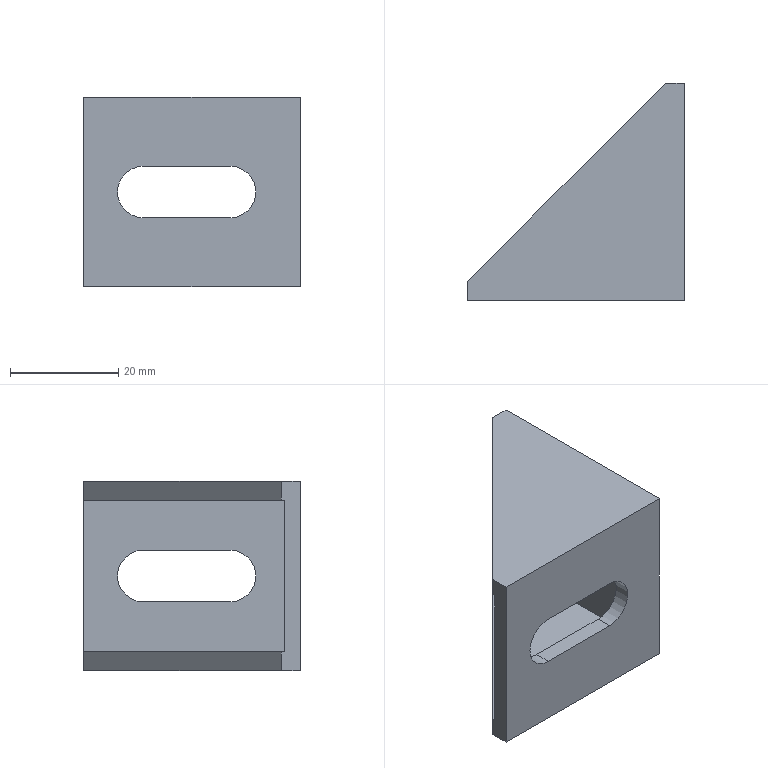Part | SolidWorks | features ICE 3, Extrusion 1 | 1 solid | 21 faces | box 40 x 40 x 35 mm | volume 11668 mm3 | plane 16 | cylinder 5 | commonest cylinder face diameters 9.5 x5
STEP:
#1=CARTESIAN_POINT('',(-16.25,0.,0.));
#2=VERTEX_POINT('',#1);
#3=CARTESIAN_POINT('',(-11.5,0.,4.75));
#4=VERTEX_POINT('',#3);
#5=CARTESIAN_POINT('',(-11.5,0.,0.));
#6=DIRECTION('',(0.,1.,0.));
#7=DIRECTION('',(-1.,0.,0.));
#8=AXIS2_PLACEMENT_3D('',#5,#6,#7);
#9=CIRCLE('',#8,4.75);
#10=EDGE_CURVE('',#2,#4,#9,.T.);
#11=ORIENTED_EDGE('',*,*,#10,.F.);
#12=CARTESIAN_POINT('',(-16.25,3.,0.));
#13=VERTEX_POINT('',#12);
#14=CARTESIAN_POINT('',(-16.25,0.,0.));
#15=DIRECTION('',(0.,1.,0.));
#16=VECTOR('',#15,1000.);
#17=LINE('',#14,#16);
#18=EDGE_CURVE('',#2,#13,#17,.T.);
#19=ORIENTED_EDGE('',*,*,#18,.T.);
#20=CARTESIAN_POINT('',(-11.5,3.,4.75));
#21=VERTEX_POINT('',#20);
#22=CARTESIAN_POINT('',(-11.5,3.,0.));
#23=DIRECTION('',(0.,1.,0.));
#24=DIRECTION('',(-1.,0.,0.));
#25=AXIS2_PLACEMENT_3D('',#22,#23,#24);
#26=CIRCLE('',#25,4.75);
#27=EDGE_CURVE('',#13,#21,#26,.T.);
#28=ORIENTED_EDGE('',*,*,#27,.T.);
#29=CARTESIAN_POINT('',(-11.5,0.,4.75));
#30=DIRECTION('',(0.,1.,0.));
#31=VECTOR('',#30,1000.);
#32=LINE('',#29,#31);
#33=EDGE_CURVE('',#4,#21,#32,.T.);
#34=ORIENTED_EDGE('',*,*,#33,.F.);
#35=EDGE_LOOP('',(#11,#19,#28,#34));
#36=FACE_OUTER_BOUND('',#35,.T.);
#37=CARTESIAN_POINT('',(-11.5,0.,0.));
#38=DIRECTION('',(0.,1.,0.));
#39=DIRECTION('',(-1.,0.,0.));
#40=AXIS2_PLACEMENT_3D('',#37,#38,#39);
#41=CYLINDRICAL_SURFACE('',#40,4.75);
#42=ADVANCED_FACE('',(#36),#41,.F.);
#43=CARTESIAN_POINT('',(14.,40.,14.));
#44=VERTEX_POINT('',#43);
#45=CARTESIAN_POINT('',(14.5,40.,14.));
#46=VERTEX_POINT('',#45);
#47=CARTESIAN_POINT('',(17.5,40.,14.));
#48=DIRECTION('',(1.,0.,0.));
#49=VECTOR('',#48,1000.);
#50=LINE('',#47,#49);
#51=EDGE_CURVE('',#44,#46,#50,.T.);
#52=ORIENTED_EDGE('',*,*,#51,.F.);
#53=CARTESIAN_POINT('',(14.,40.,17.5));
#54=VERTEX_POINT('',#53);
#55=CARTESIAN_POINT('',(14.,40.,17.5));
#56=DIRECTION('',(0.,0.,-1.));
#57=VECTOR('',#56,1000.);
#58=LINE('',#55,#57);
#59=EDGE_CURVE('',#54,#44,#58,.T.);
#60=ORIENTED_EDGE('',*,*,#59,.F.);
#61=CARTESIAN_POINT('',(17.5,40.,17.5));
#62=VERTEX_POINT('',#61);
#63=CARTESIAN_POINT('',(17.5,40.,17.5));
#64=DIRECTION('',(-1.,0.,0.));
#65=VECTOR('',#64,1000.);
#66=LINE('',#63,#65);
#67=EDGE_CURVE('',#62,#54,#66,.T.);
#68=ORIENTED_EDGE('',*,*,#67,.F.);
#69=CARTESIAN_POINT('',(17.5,40.,-17.5));
#70=VERTEX_POINT('',#69);
#71=CARTESIAN_POINT('',(17.5,40.,17.5));
#72=DIRECTION('',(0.,0.,-1.));
#73=VECTOR('',#72,1000.);
#74=LINE('',#71,#73);
#75=EDGE_CURVE('',#62,#70,#74,.T.);
#76=ORIENTED_EDGE('',*,*,#75,.T.);
#77=CARTESIAN_POINT('',(14.,40.,-17.5));
#78=VERTEX_POINT('',#77);
#79=CARTESIAN_POINT('',(17.5,40.,-17.5));
#80=DIRECTION('',(-1.,0.,0.));
#81=VECTOR('',#80,1000.);
#82=LINE('',#79,#81);
#83=EDGE_CURVE('',#70,#78,#82,.T.);
#84=ORIENTED_EDGE('',*,*,#83,.T.);
#85=CARTESIAN_POINT('',(14.,40.,-14.));
#86=VERTEX_POINT('',#85);
#87=CARTESIAN_POINT('',(14.,40.,17.5));
#88=DIRECTION('',(0.,0.,-1.));
#89=VECTOR('',#88,1000.);
#90=LINE('',#87,#89);
#91=EDGE_CURVE('',#86,#78,#90,.T.);
#92=ORIENTED_EDGE('',*,*,#91,.F.);
#93=CARTESIAN_POINT('',(14.5,40.,-14.));
#94=VERTEX_POINT('',#93);
#95=CARTESIAN_POINT('',(17.5,40.,-14.));
#96=DIRECTION('',(1.,0.,0.));
#97=VECTOR('',#96,1000.);
#98=LINE('',#95,#97);
#99=EDGE_CURVE('',#86,#94,#98,.T.);
#100=ORIENTED_EDGE('',*,*,#99,.T.);
#101=CARTESIAN_POINT('',(14.5,40.,17.5));
#102=DIRECTION('',(0.,0.,-1.));
#103=VECTOR('',#102,1000.);
#104=LINE('',#101,#103);
#105=EDGE_CURVE('',#46,#94,#104,.T.);
#106=ORIENTED_EDGE('',*,*,#105,.F.);
#107=EDGE_LOOP('',(#52,#60,#68,#76,#84,#92,#100,#106));
#108=FACE_OUTER_BOUND('',#107,.T.);
#109=CARTESIAN_POINT('',(17.5,40.,17.5));
#110=DIRECTION('',(0.,-1.,0.));
#111=DIRECTION('',(0.,0.,-1.));
#112=AXIS2_PLACEMENT_3D('',#109,#110,#111);
#113=PLANE('',#112);
#114=ADVANCED_FACE('',(#108),#113,.F.);
#115=CARTESIAN_POINT('',(-22.5,3.5,14.));
#116=VERTEX_POINT('',#115);
#117=CARTESIAN_POINT('',(14.,40.,14.));
#118=DIRECTION('',(0.7071,0.7071,0.));
#119=VECTOR('',#118,1000.);
#120=LINE('',#117,#119);
#121=EDGE_CURVE('',#116,#44,#120,.T.);
#122=ORIENTED_EDGE('',*,*,#121,.F.);
#123=CARTESIAN_POINT('',(-22.5,3.5,17.5));
#124=VERTEX_POINT('',#123);
#125=CARTESIAN_POINT('',(-22.5,3.5,17.5));
#126=DIRECTION('',(0.,0.,-1.));
#127=VECTOR('',#126,1000.);
#128=LINE('',#125,#127);
#129=EDGE_CURVE('',#124,#116,#128,.T.);
#130=ORIENTED_EDGE('',*,*,#129,.F.);
#131=CARTESIAN_POINT('',(14.,40.,17.5));
#132=DIRECTION('',(-0.7071,-0.7071,0.));
#133=VECTOR('',#132,1000.);
#134=LINE('',#131,#133);
#135=EDGE_CURVE('',#54,#124,#134,.T.);
#136=ORIENTED_EDGE('',*,*,#135,.F.);
#137=ORIENTED_EDGE('',*,*,#59,.T.);
#138=EDGE_LOOP('',(#122,#130,#136,#137));
#139=FACE_OUTER_BOUND('',#138,.T.);
#140=CARTESIAN_POINT('',(14.,40.,17.5));
#141=DIRECTION('',(0.7071,-0.7071,0.));
#142=DIRECTION('',(0.7071,0.7071,0.));
#143=AXIS2_PLACEMENT_3D('',#140,#141,#142);
#144=PLANE('',#143);
#145=ADVANCED_FACE('',(#139),#144,.F.);
#146=CARTESIAN_POINT('',(-22.5,3.,14.));
#147=VERTEX_POINT('',#146);
#148=CARTESIAN_POINT('',(-22.5,0.,14.));
#149=DIRECTION('',(0.,1.,0.));
#150=VECTOR('',#149,1000.);
#151=LINE('',#148,#150);
#152=EDGE_CURVE('',#147,#116,#151,.T.);
#153=ORIENTED_EDGE('',*,*,#152,.F.);
#154=CARTESIAN_POINT('',(-22.5,3.,-14.));
#155=VERTEX_POINT('',#154);
#156=CARTESIAN_POINT('',(-22.5,3.,17.5));
#157=DIRECTION('',(0.,0.,1.));
#158=VECTOR('',#157,1000.);
#159=LINE('',#156,#158);
#160=EDGE_CURVE('',#155,#147,#159,.T.);
#161=ORIENTED_EDGE('',*,*,#160,.F.);
#162=CARTESIAN_POINT('',(-22.5,3.5,-14.));
#163=VERTEX_POINT('',#162);
#164=CARTESIAN_POINT('',(-22.5,0.,-14.));
#165=DIRECTION('',(0.,1.,0.));
#166=VECTOR('',#165,1000.);
#167=LINE('',#164,#166);
#168=EDGE_CURVE('',#155,#163,#167,.T.);
#169=ORIENTED_EDGE('',*,*,#168,.T.);
#170=CARTESIAN_POINT('',(-22.5,3.5,-17.5));
#171=VERTEX_POINT('',#170);
#172=CARTESIAN_POINT('',(-22.5,3.5,17.5));
#173=DIRECTION('',(0.,0.,-1.));
#174=VECTOR('',#173,1000.);
#175=LINE('',#172,#174);
#176=EDGE_CURVE('',#163,#171,#175,.T.);
#177=ORIENTED_EDGE('',*,*,#176,.T.);
#178=CARTESIAN_POINT('',(-22.5,0.,-17.5));
#179=VERTEX_POINT('',#178);
#180=CARTESIAN_POINT('',(-22.5,0.,-17.5));
#181=DIRECTION('',(0.,-1.,0.));
#182=VECTOR('',#181,1000.);
#183=LINE('',#180,#182);
#184=EDGE_CURVE('',#171,#179,#183,.T.);
#185=ORIENTED_EDGE('',*,*,#184,.T.);
#186=CARTESIAN_POINT('',(-22.5,0.,17.5));
#187=VERTEX_POINT('',#186);
#188=CARTESIAN_POINT('',(-22.5,0.,17.5));
#189=DIRECTION('',(0.,0.,-1.));
#190=VECTOR('',#189,1000.);
#191=LINE('',#188,#190);
#192=EDGE_CURVE('',#187,#179,#191,.T.);
#193=ORIENTED_EDGE('',*,*,#192,.F.);
#194=CARTESIAN_POINT('',(-22.5,0.,17.5));
#195=DIRECTION('',(0.,-1.,0.));
#196=VECTOR('',#195,1000.);
#197=LINE('',#194,#196);
#198=EDGE_CURVE('',#124,#187,#197,.T.);
#199=ORIENTED_EDGE('',*,*,#198,.F.);
#200=ORIENTED_EDGE('',*,*,#129,.T.);
#201=EDGE_LOOP('',(#153,#161,#169,#177,#185,#193,#199,#200));
#202=FACE_OUTER_BOUND('',#201,.T.);
#203=CARTESIAN_POINT('',(-22.5,0.,17.5));
#204=DIRECTION('',(1.,0.,0.));
#205=DIRECTION('',(0.,0.,-1.));
#206=AXIS2_PLACEMENT_3D('',#203,#204,#205);
#207=PLANE('',#206);
#208=ADVANCED_FACE('',(#202),#207,.F.);
#209=CARTESIAN_POINT('',(17.5,29.,-4.75));
#210=VERTEX_POINT('',#209);
#211=CARTESIAN_POINT('',(17.5,13.,-4.75));
#212=VERTEX_POINT('',#211);
#213=CARTESIAN_POINT('',(17.5,13.,-4.75));
#214=DIRECTION('',(0.,-1.,0.));
#215=VECTOR('',#214,1000.);
#216=LINE('',#213,#215);
#217=EDGE_CURVE('',#210,#212,#216,.T.);
#218=ORIENTED_EDGE('',*,*,#217,.T.);
#219=CARTESIAN_POINT('',(17.5,13.,4.75));
#220=VERTEX_POINT('',#219);
#221=CARTESIAN_POINT('',(17.5,13.,0.));
#222=DIRECTION('',(-1.,0.,0.));
#223=DIRECTION('',(0.,0.,1.));
#224=AXIS2_PLACEMENT_3D('',#221,#222,#223);
#225=CIRCLE('',#224,4.75);
#226=EDGE_CURVE('',#212,#220,#225,.T.);
#227=ORIENTED_EDGE('',*,*,#226,.T.);
#228=CARTESIAN_POINT('',(17.5,29.,4.75));
#229=VERTEX_POINT('',#228);
#230=CARTESIAN_POINT('',(17.5,13.,4.75));
#231=DIRECTION('',(0.,1.,0.));
#232=VECTOR('',#231,1000.);
#233=LINE('',#230,#232);
#234=EDGE_CURVE('',#220,#229,#233,.T.);
#235=ORIENTED_EDGE('',*,*,#234,.T.);
#236=CARTESIAN_POINT('',(17.5,29.,0.));
#237=DIRECTION('',(-1.,0.,0.));
#238=DIRECTION('',(0.,0.,1.));
#239=AXIS2_PLACEMENT_3D('',#236,#237,#238);
#240=CIRCLE('',#239,4.75);
#241=EDGE_CURVE('',#229,#210,#240,.T.);
#242=ORIENTED_EDGE('',*,*,#241,.T.);
#243=EDGE_LOOP('',(#218,#227,#235,#242));
#244=FACE_BOUND('',#243,.T.);
#245=CARTESIAN_POINT('',(17.5,0.,-17.5));
#246=VERTEX_POINT('',#245);
#247=CARTESIAN_POINT('',(17.5,0.,-17.5));
#248=DIRECTION('',(0.,1.,0.));
#249=VECTOR('',#248,1000.);
#250=LINE('',#247,#249);
#251=EDGE_CURVE('',#246,#70,#250,.T.);
#252=ORIENTED_EDGE('',*,*,#251,.T.);
#253=ORIENTED_EDGE('',*,*,#75,.F.);
#254=CARTESIAN_POINT('',(17.5,0.,17.5));
#255=VERTEX_POINT('',#254);
#256=CARTESIAN_POINT('',(17.5,0.,17.5));
#257=DIRECTION('',(0.,1.,0.));
#258=VECTOR('',#257,1000.);
#259=LINE('',#256,#258);
#260=EDGE_CURVE('',#255,#62,#259,.T.);
#261=ORIENTED_EDGE('',*,*,#260,.F.);
#262=CARTESIAN_POINT('',(17.5,0.,17.5));
#263=DIRECTION('',(0.,0.,-1.));
#264=VECTOR('',#263,1000.);
#265=LINE('',#262,#264);
#266=EDGE_CURVE('',#255,#246,#265,.T.);
#267=ORIENTED_EDGE('',*,*,#266,.T.);
#268=EDGE_LOOP('',(#252,#253,#261,#267));
#269=FACE_OUTER_BOUND('',#268,.T.);
#270=CARTESIAN_POINT('',(17.5,0.,17.5));
#271=DIRECTION('',(-1.,0.,0.));
#272=DIRECTION('',(0.,0.,1.));
#273=AXIS2_PLACEMENT_3D('',#270,#271,#272);
#274=PLANE('',#273);
#275=ADVANCED_FACE('',(#244,#269),#274,.F.);
#276=ORIENTED_EDGE('',*,*,#176,.F.);
#277=CARTESIAN_POINT('',(14.,40.,-14.));
#278=DIRECTION('',(0.7071,0.7071,0.));
#279=VECTOR('',#278,1000.);
#280=LINE('',#277,#279);
#281=EDGE_CURVE('',#163,#86,#280,.T.);
#282=ORIENTED_EDGE('',*,*,#281,.T.);
#283=ORIENTED_EDGE('',*,*,#91,.T.);
#284=CARTESIAN_POINT('',(14.,40.,-17.5));
#285=DIRECTION('',(-0.7071,-0.7071,0.));
#286=VECTOR('',#285,1000.);
#287=LINE('',#284,#286);
#288=EDGE_CURVE('',#78,#171,#287,.T.);
#289=ORIENTED_EDGE('',*,*,#288,.T.);
#290=EDGE_LOOP('',(#276,#282,#283,#289));
#291=FACE_OUTER_BOUND('',#290,.T.);
#292=CARTESIAN_POINT('',(14.,40.,17.5));
#293=DIRECTION('',(0.7071,-0.7071,0.));
#294=DIRECTION('',(0.7071,0.7071,0.));
#295=AXIS2_PLACEMENT_3D('',#292,#293,#294);
#296=PLANE('',#295);
#297=ADVANCED_FACE('',(#291),#296,.F.);
#298=CARTESIAN_POINT('',(4.5,0.,-4.75));
#299=VERTEX_POINT('',#298);
#300=CARTESIAN_POINT('',(-11.5,0.,-4.75));
#301=VERTEX_POINT('',#300);
#302=CARTESIAN_POINT('',(-11.5,0.,-4.75));
#303=DIRECTION('',(-1.,0.,0.));
#304=VECTOR('',#303,1000.);
#305=LINE('',#302,#304);
#306=EDGE_CURVE('',#299,#301,#305,.T.);
#307=ORIENTED_EDGE('',*,*,#306,.T.);
#308=CARTESIAN_POINT('',(-11.5,0.,0.));
#309=DIRECTION('',(0.,1.,0.));
#310=DIRECTION('',(-1.,0.,0.));
#311=AXIS2_PLACEMENT_3D('',#308,#309,#310);
#312=CIRCLE('',#311,4.75);
#313=EDGE_CURVE('',#301,#2,#312,.T.);
#314=ORIENTED_EDGE('',*,*,#313,.T.);
#315=ORIENTED_EDGE('',*,*,#10,.T.);
#316=CARTESIAN_POINT('',(4.5,0.,4.75));
#317=VERTEX_POINT('',#316);
#318=CARTESIAN_POINT('',(-11.5,0.,4.75));
#319=DIRECTION('',(1.,0.,0.));
#320=VECTOR('',#319,1000.);
#321=LINE('',#318,#320);
#322=EDGE_CURVE('',#4,#317,#321,.T.);
#323=ORIENTED_EDGE('',*,*,#322,.T.);
#324=CARTESIAN_POINT('',(4.5,0.,0.));
#325=DIRECTION('',(0.,1.,0.));
#326=DIRECTION('',(-1.,0.,0.));
#327=AXIS2_PLACEMENT_3D('',#324,#325,#326);
#328=CIRCLE('',#327,4.75);
#329=EDGE_CURVE('',#317,#299,#328,.T.);
#330=ORIENTED_EDGE('',*,*,#329,.T.);
#331=EDGE_LOOP('',(#307,#314,#315,#323,#330));
#332=FACE_BOUND('',#331,.T.);
#333=CARTESIAN_POINT('',(-22.5,0.,-17.5));
#334=DIRECTION('',(1.,0.,0.));
#335=VECTOR('',#334,1000.);
#336=LINE('',#333,#335);
#337=EDGE_CURVE('',#179,#246,#336,.T.);
#338=ORIENTED_EDGE('',*,*,#337,.T.);
#339=ORIENTED_EDGE('',*,*,#266,.F.);
#340=CARTESIAN_POINT('',(-22.5,0.,17.5));
#341=DIRECTION('',(1.,0.,0.));
#342=VECTOR('',#341,1000.);
#343=LINE('',#340,#342);
#344=EDGE_CURVE('',#187,#255,#343,.T.);
#345=ORIENTED_EDGE('',*,*,#344,.F.);
#346=ORIENTED_EDGE('',*,*,#192,.T.);
#347=EDGE_LOOP('',(#338,#339,#345,#346));
#348=FACE_OUTER_BOUND('',#347,.T.);
#349=CARTESIAN_POINT('',(-22.5,0.,17.5));
#350=DIRECTION('',(0.,1.,0.));
#351=DIRECTION('',(0.,0.,1.));
#352=AXIS2_PLACEMENT_3D('',#349,#350,#351);
#353=PLANE('',#352);
#354=ADVANCED_FACE('',(#332,#348),#353,.F.);
#355=ORIENTED_EDGE('',*,*,#260,.T.);
#356=ORIENTED_EDGE('',*,*,#67,.T.);
#357=ORIENTED_EDGE('',*,*,#135,.T.);
#358=ORIENTED_EDGE('',*,*,#198,.T.);
#359=ORIENTED_EDGE('',*,*,#344,.T.);
#360=EDGE_LOOP('',(#355,#356,#357,#358,#359));
#361=FACE_OUTER_BOUND('',#360,.T.);
#362=CARTESIAN_POINT('',(0.,0.,17.5));
#363=DIRECTION('',(0.,0.,1.));
#364=DIRECTION('',(1.,0.,0.));
#365=AXIS2_PLACEMENT_3D('',#362,#363,#364);
#366=PLANE('',#365);
#367=ADVANCED_FACE('',(#361),#366,.T.);
#368=ORIENTED_EDGE('',*,*,#251,.F.);
#369=ORIENTED_EDGE('',*,*,#337,.F.);
#370=ORIENTED_EDGE('',*,*,#184,.F.);
#371=ORIENTED_EDGE('',*,*,#288,.F.);
#372=ORIENTED_EDGE('',*,*,#83,.F.);
#373=EDGE_LOOP('',(#368,#369,#370,#371,#372));
#374=FACE_OUTER_BOUND('',#373,.T.);
#375=CARTESIAN_POINT('',(0.,0.,-17.5));
#376=DIRECTION('',(0.,0.,1.));
#377=DIRECTION('',(1.,0.,0.));
#378=AXIS2_PLACEMENT_3D('',#375,#376,#377);
#379=PLANE('',#378);
#380=ADVANCED_FACE('',(#374),#379,.F.);
#381=CARTESIAN_POINT('',(14.5,13.,-4.75));
#382=VERTEX_POINT('',#381);
#383=CARTESIAN_POINT('',(14.5,13.,4.75));
#384=VERTEX_POINT('',#383);
#385=CARTESIAN_POINT('',(14.5,13.,0.));
#386=DIRECTION('',(-1.,0.,0.));
#387=DIRECTION('',(0.,0.,1.));
#388=AXIS2_PLACEMENT_3D('',#385,#386,#387);
#389=CIRCLE('',#388,4.75);
#390=EDGE_CURVE('',#382,#384,#389,.T.);
#391=ORIENTED_EDGE('',*,*,#390,.F.);
#392=CARTESIAN_POINT('',(14.5,29.,-4.75));
#393=VERTEX_POINT('',#392);
#394=CARTESIAN_POINT('',(14.5,13.,-4.75));
#395=DIRECTION('',(0.,-1.,0.));
#396=VECTOR('',#395,1000.);
#397=LINE('',#394,#396);
#398=EDGE_CURVE('',#393,#382,#397,.T.);
#399=ORIENTED_EDGE('',*,*,#398,.F.);
#400=CARTESIAN_POINT('',(14.5,29.,4.75));
#401=VERTEX_POINT('',#400);
#402=CARTESIAN_POINT('',(14.5,29.,0.));
#403=DIRECTION('',(-1.,0.,0.));
#404=DIRECTION('',(0.,0.,1.));
#405=AXIS2_PLACEMENT_3D('',#402,#403,#404);
#406=CIRCLE('',#405,4.75);
#407=EDGE_CURVE('',#401,#393,#406,.T.);
#408=ORIENTED_EDGE('',*,*,#407,.F.);
#409=CARTESIAN_POINT('',(14.5,13.,4.75));
#410=DIRECTION('',(0.,1.,0.));
#411=VECTOR('',#410,1000.);
#412=LINE('',#409,#411);
#413=EDGE_CURVE('',#384,#401,#412,.T.);
#414=ORIENTED_EDGE('',*,*,#413,.F.);
#415=EDGE_LOOP('',(#391,#399,#408,#414));
#416=FACE_BOUND('',#415,.T.);
#417=ORIENTED_EDGE('',*,*,#105,.T.);
#418=CARTESIAN_POINT('',(14.5,3.,-14.));
#419=VERTEX_POINT('',#418);
#420=CARTESIAN_POINT('',(14.5,3.,-14.));
#421=DIRECTION('',(0.,1.,0.));
#422=VECTOR('',#421,1000.);
#423=LINE('',#420,#422);
#424=EDGE_CURVE('',#419,#94,#423,.T.);
#425=ORIENTED_EDGE('',*,*,#424,.F.);
#426=CARTESIAN_POINT('',(14.5,3.,14.));
#427=VERTEX_POINT('',#426);
#428=CARTESIAN_POINT('',(14.5,3.,14.));
#429=DIRECTION('',(0.,0.,-1.));
#430=VECTOR('',#429,1000.);
#431=LINE('',#428,#430);
#432=EDGE_CURVE('',#427,#419,#431,.T.);
#433=ORIENTED_EDGE('',*,*,#432,.F.);
#434=CARTESIAN_POINT('',(14.5,3.,14.));
#435=DIRECTION('',(0.,1.,0.));
#436=VECTOR('',#435,1000.);
#437=LINE('',#434,#436);
#438=EDGE_CURVE('',#427,#46,#437,.T.);
#439=ORIENTED_EDGE('',*,*,#438,.T.);
#440=EDGE_LOOP('',(#417,#425,#433,#439));
#441=FACE_OUTER_BOUND('',#440,.T.);
#442=CARTESIAN_POINT('',(14.5,3.,14.));
#443=DIRECTION('',(-1.,0.,0.));
#444=DIRECTION('',(0.,0.,1.));
#445=AXIS2_PLACEMENT_3D('',#442,#443,#444);
#446=PLANE('',#445);
#447=ADVANCED_FACE('',(#416,#441),#446,.T.);
#448=CARTESIAN_POINT('',(-11.5,3.,-4.75));
#449=VERTEX_POINT('',#448);
#450=CARTESIAN_POINT('',(-11.5,3.,0.));
#451=DIRECTION('',(0.,1.,0.));
#452=DIRECTION('',(-1.,0.,0.));
#453=AXIS2_PLACEMENT_3D('',#450,#451,#452);
#454=CIRCLE('',#453,4.75);
#455=EDGE_CURVE('',#449,#13,#454,.T.);
#456=ORIENTED_EDGE('',*,*,#455,.F.);
#457=CARTESIAN_POINT('',(4.5,3.,-4.75));
#458=VERTEX_POINT('',#457);
#459=CARTESIAN_POINT('',(-11.5,3.,-4.75));
#460=DIRECTION('',(-1.,0.,0.));
#461=VECTOR('',#460,1000.);
#462=LINE('',#459,#461);
#463=EDGE_CURVE('',#458,#449,#462,.T.);
#464=ORIENTED_EDGE('',*,*,#463,.F.);
#465=CARTESIAN_POINT('',(4.5,3.,4.75));
#466=VERTEX_POINT('',#465);
#467=CARTESIAN_POINT('',(4.5,3.,0.));
#468=DIRECTION('',(0.,1.,0.));
#469=DIRECTION('',(-1.,0.,0.));
#470=AXIS2_PLACEMENT_3D('',#467,#468,#469);
#471=CIRCLE('',#470,4.75);
#472=EDGE_CURVE('',#466,#458,#471,.T.);
#473=ORIENTED_EDGE('',*,*,#472,.F.);
#474=CARTESIAN_POINT('',(-11.5,3.,4.75));
#475=DIRECTION('',(1.,0.,0.));
#476=VECTOR('',#475,1000.);
#477=LINE('',#474,#476);
#478=EDGE_CURVE('',#21,#466,#477,.T.);
#479=ORIENTED_EDGE('',*,*,#478,.F.);
#480=ORIENTED_EDGE('',*,*,#27,.F.);
#481=EDGE_LOOP('',(#456,#464,#473,#479,#480));
#482=FACE_BOUND('',#481,.T.);
#483=ORIENTED_EDGE('',*,*,#160,.T.);
#484=CARTESIAN_POINT('',(-34.195,3.,14.));
#485=DIRECTION('',(1.,0.,0.));
#486=VECTOR('',#485,1000.);
#487=LINE('',#484,#486);
#488=EDGE_CURVE('',#147,#427,#487,.T.);
#489=ORIENTED_EDGE('',*,*,#488,.T.);
#490=ORIENTED_EDGE('',*,*,#432,.T.);
#491=CARTESIAN_POINT('',(-34.195,3.,-14.));
#492=DIRECTION('',(1.,0.,0.));
#493=VECTOR('',#492,1000.);
#494=LINE('',#491,#493);
#495=EDGE_CURVE('',#155,#419,#494,.T.);
#496=ORIENTED_EDGE('',*,*,#495,.F.);
#497=EDGE_LOOP('',(#483,#489,#490,#496));
#498=FACE_OUTER_BOUND('',#497,.T.);
#499=CARTESIAN_POINT('',(-34.195,3.,14.));
#500=DIRECTION('',(0.,1.,0.));
#501=DIRECTION('',(-1.,0.,0.));
#502=AXIS2_PLACEMENT_3D('',#499,#500,#501);
#503=PLANE('',#502);
#504=ADVANCED_FACE('',(#482,#498),#503,.T.);
#505=ORIENTED_EDGE('',*,*,#51,.T.);
#506=ORIENTED_EDGE('',*,*,#438,.F.);
#507=ORIENTED_EDGE('',*,*,#488,.F.);
#508=ORIENTED_EDGE('',*,*,#152,.T.);
#509=ORIENTED_EDGE('',*,*,#121,.T.);
#510=EDGE_LOOP('',(#505,#506,#507,#508,#509));
#511=FACE_OUTER_BOUND('',#510,.T.);
#512=CARTESIAN_POINT('',(0.,0.,14.));
#513=DIRECTION('',(0.,0.,-1.));
#514=DIRECTION('',(-1.,0.,0.));
#515=AXIS2_PLACEMENT_3D('',#512,#513,#514);
#516=PLANE('',#515);
#517=ADVANCED_FACE('',(#511),#516,.T.);
#518=ORIENTED_EDGE('',*,*,#281,.F.);
#519=ORIENTED_EDGE('',*,*,#168,.F.);
#520=ORIENTED_EDGE('',*,*,#495,.T.);
#521=ORIENTED_EDGE('',*,*,#424,.T.);
#522=ORIENTED_EDGE('',*,*,#99,.F.);
#523=EDGE_LOOP('',(#518,#519,#520,#521,#522));
#524=FACE_OUTER_BOUND('',#523,.T.);
#525=CARTESIAN_POINT('',(0.,0.,-14.));
#526=DIRECTION('',(0.,0.,-1.));
#527=DIRECTION('',(-1.,0.,0.));
#528=AXIS2_PLACEMENT_3D('',#525,#526,#527);
#529=PLANE('',#528);
#530=ADVANCED_FACE('',(#524),#529,.F.);
#531=ORIENTED_EDGE('',*,*,#18,.F.);
#532=ORIENTED_EDGE('',*,*,#313,.F.);
#533=CARTESIAN_POINT('',(-11.5,0.,-4.75));
#534=DIRECTION('',(0.,1.,0.));
#535=VECTOR('',#534,1000.);
#536=LINE('',#533,#535);
#537=EDGE_CURVE('',#301,#449,#536,.T.);
#538=ORIENTED_EDGE('',*,*,#537,.T.);
#539=ORIENTED_EDGE('',*,*,#455,.T.);
#540=EDGE_LOOP('',(#531,#532,#538,#539));
#541=FACE_OUTER_BOUND('',#540,.T.);
#542=CARTESIAN_POINT('',(-11.5,0.,0.));
#543=DIRECTION('',(0.,1.,0.));
#544=DIRECTION('',(-1.,0.,0.));
#545=AXIS2_PLACEMENT_3D('',#542,#543,#544);
#546=CYLINDRICAL_SURFACE('',#545,4.75);
#547=ADVANCED_FACE('',(#541),#546,.F.);
#548=ORIENTED_EDGE('',*,*,#463,.T.);
#549=ORIENTED_EDGE('',*,*,#537,.F.);
#550=ORIENTED_EDGE('',*,*,#306,.F.);
#551=CARTESIAN_POINT('',(4.5,0.,-4.75));
#552=DIRECTION('',(0.,1.,0.));
#553=VECTOR('',#552,1000.);
#554=LINE('',#551,#553);
#555=EDGE_CURVE('',#299,#458,#554,.T.);
#556=ORIENTED_EDGE('',*,*,#555,.T.);
#557=EDGE_LOOP('',(#548,#549,#550,#556));
#558=FACE_OUTER_BOUND('',#557,.T.);
#559=CARTESIAN_POINT('',(-11.5,0.,-4.75));
#560=DIRECTION('',(0.,0.,-1.));
#561=DIRECTION('',(-1.,0.,0.));
#562=AXIS2_PLACEMENT_3D('',#559,#560,#561);
#563=PLANE('',#562);
#564=ADVANCED_FACE('',(#558),#563,.F.);
#565=ORIENTED_EDGE('',*,*,#472,.T.);
#566=ORIENTED_EDGE('',*,*,#555,.F.);
#567=ORIENTED_EDGE('',*,*,#329,.F.);
#568=CARTESIAN_POINT('',(4.5,0.,4.75));
#569=DIRECTION('',(0.,1.,0.));
#570=VECTOR('',#569,1000.);
#571=LINE('',#568,#570);
#572=EDGE_CURVE('',#317,#466,#571,.T.);
#573=ORIENTED_EDGE('',*,*,#572,.T.);
#574=EDGE_LOOP('',(#565,#566,#567,#573));
#575=FACE_OUTER_BOUND('',#574,.T.);
#576=CARTESIAN_POINT('',(4.5,0.,0.));
#577=DIRECTION('',(0.,1.,0.));
#578=DIRECTION('',(-1.,0.,0.));
#579=AXIS2_PLACEMENT_3D('',#576,#577,#578);
#580=CYLINDRICAL_SURFACE('',#579,4.75);
#581=ADVANCED_FACE('',(#575),#580,.F.);
#582=ORIENTED_EDGE('',*,*,#478,.T.);
#583=ORIENTED_EDGE('',*,*,#572,.F.);
#584=ORIENTED_EDGE('',*,*,#322,.F.);
#585=ORIENTED_EDGE('',*,*,#33,.T.);
#586=EDGE_LOOP('',(#582,#583,#584,#585));
#587=FACE_OUTER_BOUND('',#586,.T.);
#588=CARTESIAN_POINT('',(-11.5,0.,4.75));
#589=DIRECTION('',(0.,0.,1.));
#590=DIRECTION('',(1.,0.,0.));
#591=AXIS2_PLACEMENT_3D('',#588,#589,#590);
#592=PLANE('',#591);
#593=ADVANCED_FACE('',(#587),#592,.F.);
#594=ORIENTED_EDGE('',*,*,#390,.T.);
#595=CARTESIAN_POINT('',(17.5,13.,4.75));
#596=DIRECTION('',(-1.,0.,0.));
#597=VECTOR('',#596,1000.);
#598=LINE('',#595,#597);
#599=EDGE_CURVE('',#220,#384,#598,.T.);
#600=ORIENTED_EDGE('',*,*,#599,.F.);
#601=ORIENTED_EDGE('',*,*,#226,.F.);
#602=CARTESIAN_POINT('',(17.5,13.,-4.75));
#603=DIRECTION('',(-1.,0.,0.));
#604=VECTOR('',#603,1000.);
#605=LINE('',#602,#604);
#606=EDGE_CURVE('',#212,#382,#605,.T.);
#607=ORIENTED_EDGE('',*,*,#606,.T.);
#608=EDGE_LOOP('',(#594,#600,#601,#607));
#609=FACE_OUTER_BOUND('',#608,.T.);
#610=CARTESIAN_POINT('',(17.5,13.,0.));
#611=DIRECTION('',(-1.,0.,0.));
#612=DIRECTION('',(0.,0.,1.));
#613=AXIS2_PLACEMENT_3D('',#610,#611,#612);
#614=CYLINDRICAL_SURFACE('',#613,4.75);
#615=ADVANCED_FACE('',(#609),#614,.F.);
#616=ORIENTED_EDGE('',*,*,#398,.T.);
#617=ORIENTED_EDGE('',*,*,#606,.F.);
#618=ORIENTED_EDGE('',*,*,#217,.F.);
#619=CARTESIAN_POINT('',(17.5,29.,-4.75));
#620=DIRECTION('',(-1.,0.,0.));
#621=VECTOR('',#620,1000.);
#622=LINE('',#619,#621);
#623=EDGE_CURVE('',#210,#393,#622,.T.);
#624=ORIENTED_EDGE('',*,*,#623,.T.);
#625=EDGE_LOOP('',(#616,#617,#618,#624));
#626=FACE_OUTER_BOUND('',#625,.T.);
#627=CARTESIAN_POINT('',(17.5,13.,-4.75));
#628=DIRECTION('',(0.,0.,-1.));
#629=DIRECTION('',(-1.,0.,0.));
#630=AXIS2_PLACEMENT_3D('',#627,#628,#629);
#631=PLANE('',#630);
#632=ADVANCED_FACE('',(#626),#631,.F.);
#633=ORIENTED_EDGE('',*,*,#407,.T.);
#634=ORIENTED_EDGE('',*,*,#623,.F.);
#635=ORIENTED_EDGE('',*,*,#241,.F.);
#636=CARTESIAN_POINT('',(17.5,29.,4.75));
#637=DIRECTION('',(-1.,0.,0.));
#638=VECTOR('',#637,1000.);
#639=LINE('',#636,#638);
#640=EDGE_CURVE('',#229,#401,#639,.T.);
#641=ORIENTED_EDGE('',*,*,#640,.T.);
#642=EDGE_LOOP('',(#633,#634,#635,#641));
#643=FACE_OUTER_BOUND('',#642,.T.);
#644=CARTESIAN_POINT('',(17.5,29.,0.));
#645=DIRECTION('',(-1.,0.,0.));
#646=DIRECTION('',(0.,0.,1.));
#647=AXIS2_PLACEMENT_3D('',#644,#645,#646);
#648=CYLINDRICAL_SURFACE('',#647,4.75);
#649=ADVANCED_FACE('',(#643),#648,.F.);
#650=ORIENTED_EDGE('',*,*,#413,.T.);
#651=ORIENTED_EDGE('',*,*,#640,.F.);
#652=ORIENTED_EDGE('',*,*,#234,.F.);
#653=ORIENTED_EDGE('',*,*,#599,.T.);
#654=EDGE_LOOP('',(#650,#651,#652,#653));
#655=FACE_OUTER_BOUND('',#654,.T.);
#656=CARTESIAN_POINT('',(17.5,13.,4.75));
#657=DIRECTION('',(0.,0.,1.));
#658=DIRECTION('',(1.,0.,0.));
#659=AXIS2_PLACEMENT_3D('',#656,#657,#658);
#660=PLANE('',#659);
#661=ADVANCED_FACE('',(#655),#660,.F.);
#662=CLOSED_SHELL('',(#42,#114,#145,#208,#275,#297,#354,#367,#380,#447,#504,#517,#530,#547,#564,#581,#593,#615,#632,#649,#661));
#663=MANIFOLD_SOLID_BREP('',#662);
#664=CARTESIAN_POINT('',(0.,0.,0.));
#665=DIRECTION('',(0.,0.,1.));
#666=DIRECTION('',(1.,0.,0.));
#667=AXIS2_PLACEMENT_3D('',#664,#665,#666);
#668=(LENGTH_UNIT()NAMED_UNIT(*)SI_UNIT(.MILLI.,.METRE.));
#669=UNCERTAINTY_MEASURE_WITH_UNIT(LENGTH_MEASURE(0.00001),#668,'','');
#670=(NAMED_UNIT(*)PLANE_ANGLE_UNIT()SI_UNIT($,.RADIAN.));
#671=(NAMED_UNIT(*)SI_UNIT($,.STERADIAN.)SOLID_ANGLE_UNIT());
#672=(GEOMETRIC_REPRESENTATION_CONTEXT(3)GLOBAL_UNCERTAINTY_ASSIGNED_CONTEXT((#669))GLOBAL_UNIT_ASSIGNED_CONTEXT((#668,#670,#671))REPRESENTATION_CONTEXT('',''));
#673=ADVANCED_BREP_SHAPE_REPRESENTATION('',(#663,#667),#672);